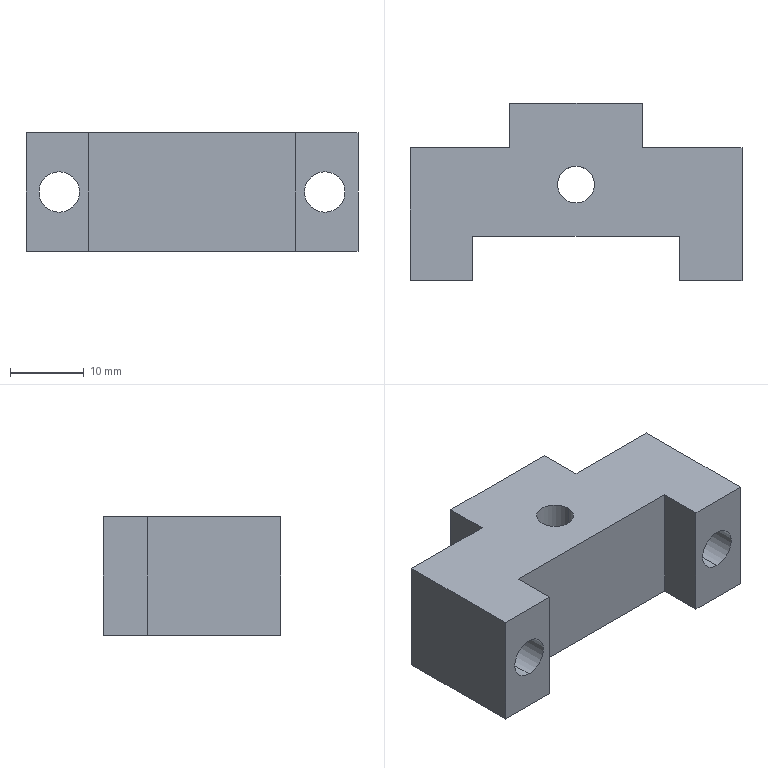Part | STEP file | BU-C02 | 1 solid | 20 faces | box 45 x 24 x 16 mm | volume 10831 mm3 | plane 14 | cylinder 6 | commonest cylinder face diameters 5.5 x4 5 x2